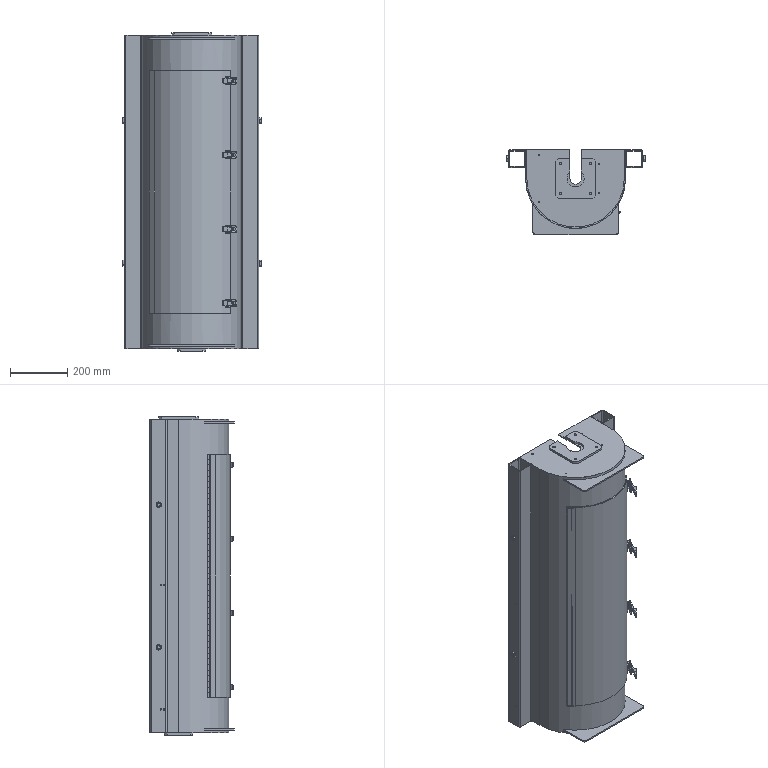Part | SolidWorks | features ReferencePattern 3, LocalLPattern 1 | 35 solids | 1520 faces | box 487 x 297 x 1116 mm | volume 6337881 mm3 | cylinder 715 | plane 697 | cone 60 | torus 48 | commonest cylinder face diameters 6.5 x129 4 x104 3.5 x88 4.2 x76 4.4 x48 5 x24